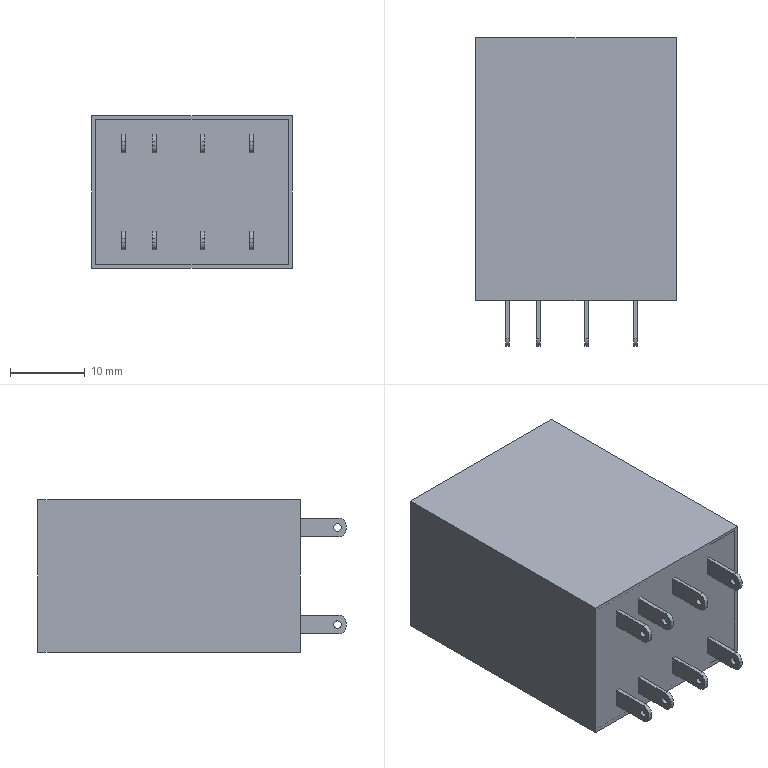Part | STEP file | Relay 1 | 1 solid | 84 faces | box 26.8 x 41.2 x 20.4 mm | volume 1978 mm3 | plane 52 | cylinder 32 | commonest cylinder face diameters 1.006 x16 2 x16